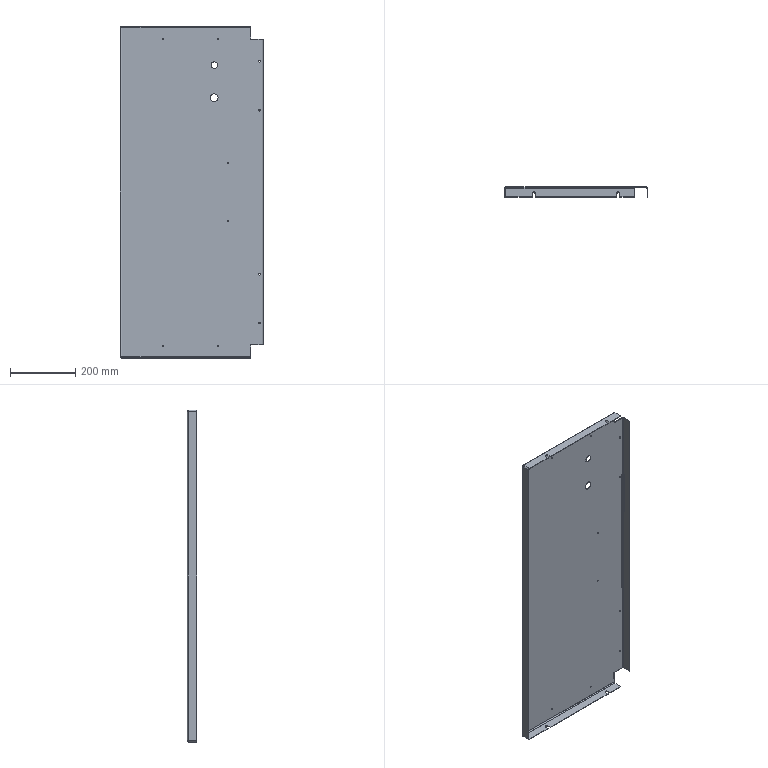Part | STEP file | 1 solid | 76 faces | box 440 x 30 x 1018 mm | volume 774968 mm3 | cylinder 40 | plane 28 | cone 4 | spline 4 | commonest cylinder face diameters 3.3 x12 5.5 x8 7 x6 10 x6 9 x4 20 x2